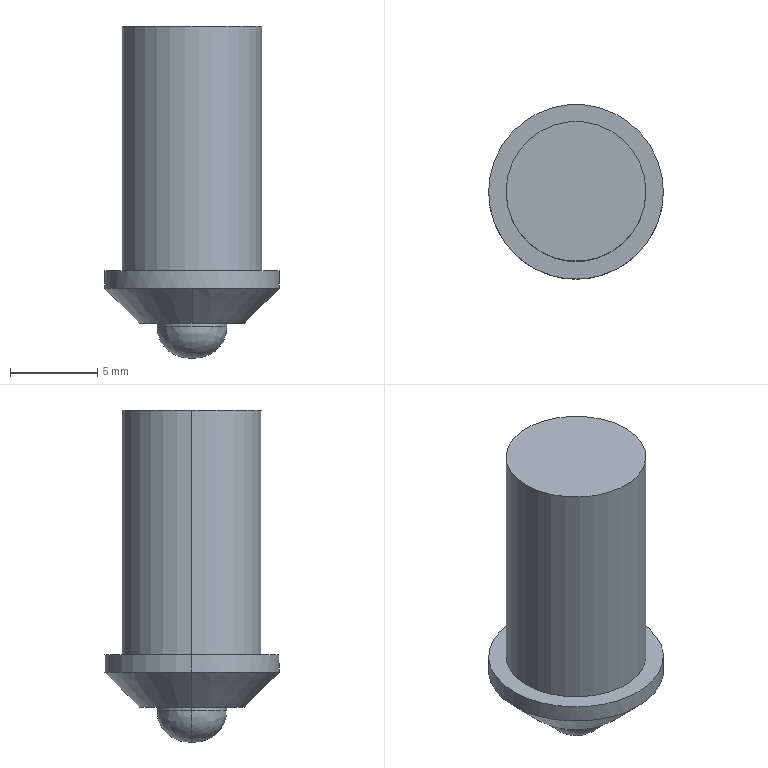Part | STEP file | 15V-DIANYUANZHISHIDENG.stp.STEP | 1 solid | 15 faces | box 10 x 10 x 19 mm | volume 903.03 mm3 | cylinder 6 | plane 4 | cone 3 | spline 2 | commonest cylinder face diameters 4 x2 8 x2 10 x2
STEP:
#1=CARTESIAN_POINT('',(0.2,0.,0.));
#2=VERTEX_POINT('',#1);
#3=CARTESIAN_POINT('',(-0.2,0.,0.));
#4=VERTEX_POINT('',#3);
#5=CARTESIAN_POINT('',(0.,0.,0.));
#6=DIRECTION('',(0.,0.,-1.));
#7=DIRECTION('',(1.,0.,0.));
#8=AXIS2_PLACEMENT_3D('',#5,#6,#7);
#9=CIRCLE('',#8,0.2);
#10=EDGE_CURVE('',#2,#4,#9,.T.);
#11=ORIENTED_EDGE('',*,*,#10,.T.);
#12=CARTESIAN_POINT('',(0.,0.,0.));
#13=DIRECTION('',(0.,0.,-1.));
#14=DIRECTION('',(-1.,0.,0.));
#15=AXIS2_PLACEMENT_3D('',#12,#13,#14);
#16=CIRCLE('',#15,0.2);
#17=EDGE_CURVE('',#4,#2,#16,.T.);
#18=ORIENTED_EDGE('',*,*,#17,.T.);
#19=EDGE_LOOP('',(#11,#18));
#20=FACE_OUTER_BOUND('',#19,.T.);
#21=CARTESIAN_POINT('',(0.,0.,0.));
#22=DIRECTION('',(0.,0.,1.));
#23=DIRECTION('',(1.,0.,0.));
#24=AXIS2_PLACEMENT_3D('',#21,#22,#23);
#25=PLANE('',#24);
#26=ADVANCED_FACE('',(#20),#25,.F.);
#27=CARTESIAN_POINT('',(-2.,0.,1.8));
#28=VERTEX_POINT('',#27);
#29=CARTESIAN_POINT('',(-0.2,0.,1.8));
#30=DIRECTION('',(0.,1.,0.));
#31=DIRECTION('',(0.,0.,-1.));
#32=AXIS2_PLACEMENT_3D('',#29,#30,#31);
#33=CIRCLE('',#32,1.8);
#34=EDGE_CURVE('',#4,#28,#33,.T.);
#35=ORIENTED_EDGE('',*,*,#34,.T.);
#36=CARTESIAN_POINT('',(2.,0.,1.8));
#37=VERTEX_POINT('',#36);
#38=CARTESIAN_POINT('',(0.,0.,1.8));
#39=DIRECTION('',(0.,0.,-1.));
#40=DIRECTION('',(-1.,0.,0.));
#41=AXIS2_PLACEMENT_3D('',#38,#39,#40);
#42=CIRCLE('',#41,2.);
#43=EDGE_CURVE('',#28,#37,#42,.T.);
#44=ORIENTED_EDGE('',*,*,#43,.T.);
#45=CARTESIAN_POINT('',(0.2,0.,1.8));
#46=DIRECTION('',(0.,-1.,0.));
#47=DIRECTION('',(0.,0.,-1.));
#48=AXIS2_PLACEMENT_3D('',#45,#46,#47);
#49=CIRCLE('',#48,1.8);
#50=EDGE_CURVE('',#2,#37,#49,.T.);
#51=ORIENTED_EDGE('',*,*,#50,.F.);
#52=ORIENTED_EDGE('',*,*,#17,.F.);
#53=EDGE_LOOP('',(#35,#44,#51,#52));
#54=FACE_OUTER_BOUND('',#53,.T.);
#55=CARTESIAN_POINT('',(0.142,-0.02032,0.0008882));
#56=CARTESIAN_POINT('',(1.238,-0.1771,-0.03391));
#57=CARTESIAN_POINT('',(2.013,-0.2881,0.7494));
#58=CARTESIAN_POINT('',(1.979,-0.2831,1.857));
#59=CARTESIAN_POINT('',(0.1553,0.07257,0.0008882));
#60=CARTESIAN_POINT('',(1.354,0.6326,-0.03391));
#61=CARTESIAN_POINT('',(2.202,1.029,0.7494));
#62=CARTESIAN_POINT('',(2.164,1.011,1.857));
#63=CARTESIAN_POINT('',(0.09383,0.1435,0.0008882));
#64=CARTESIAN_POINT('',(0.818,1.251,-0.03391));
#65=CARTESIAN_POINT('',(1.33,2.034,0.7494));
#66=CARTESIAN_POINT('',(1.308,1.999,1.857));
#67=CARTESIAN_POINT('',(0.000000002,0.1435,0.0008882));
#68=CARTESIAN_POINT('',(0.000000017,1.251,-0.03391));
#69=CARTESIAN_POINT('',(0.000000028,2.034,0.7494));
#70=CARTESIAN_POINT('',(0.000000028,1.999,1.857));
#71=CARTESIAN_POINT('',(-0.09383,0.1435,0.0008882));
#72=CARTESIAN_POINT('',(-0.818,1.251,-0.03391));
#73=CARTESIAN_POINT('',(-1.33,2.034,0.7494));
#74=CARTESIAN_POINT('',(-1.308,1.999,1.857));
#75=CARTESIAN_POINT('',(-0.1553,0.07257,0.0008882));
#76=CARTESIAN_POINT('',(-1.354,0.6326,-0.03391));
#77=CARTESIAN_POINT('',(-2.202,1.029,0.7494));
#78=CARTESIAN_POINT('',(-2.164,1.011,1.857));
#79=CARTESIAN_POINT('',(-0.142,-0.02032,0.0008882));
#80=CARTESIAN_POINT('',(-1.238,-0.1771,-0.03391));
#81=CARTESIAN_POINT('',(-2.013,-0.2881,0.7494));
#82=CARTESIAN_POINT('',(-1.979,-0.2831,1.857));
#83=(BOUNDED_SURFACE()B_SPLINE_SURFACE(3,3,((#55,#56,#57,#58),(#59,#60,#61,#62),(#63,#64,#65,#66),(#67,#68,#69,#70),(#71,#72,#73,#74),(#75,#76,#77,#78),(#79,#80,#81,#82)),.UNSPECIFIED.,.F.,.F.,.F.)B_SPLINE_SURFACE_WITH_KNOTS((4,3,4),(4,4),(0.,1.,2.),(0.,1.),.UNSPECIFIED.)GEOMETRIC_REPRESENTATION_ITEM()RATIONAL_B_SPLINE_SURFACE(((1.435,1.133,1.133,1.435),(1.105,0.8725,0.8725,1.105),(1.105,0.8725,0.8725,1.105),(1.435,1.133,1.133,1.435),(1.105,0.8725,0.8725,1.105),(1.105,0.8725,0.8725,1.105),(1.435,1.133,1.133,1.435)))REPRESENTATION_ITEM('')SURFACE());
#84=ADVANCED_FACE('',(#54),#83,.T.);
#85=ORIENTED_EDGE('',*,*,#50,.T.);
#86=CARTESIAN_POINT('',(0.,0.,1.8));
#87=DIRECTION('',(0.,0.,-1.));
#88=DIRECTION('',(1.,0.,0.));
#89=AXIS2_PLACEMENT_3D('',#86,#87,#88);
#90=CIRCLE('',#89,2.);
#91=EDGE_CURVE('',#37,#28,#90,.T.);
#92=ORIENTED_EDGE('',*,*,#91,.T.);
#93=ORIENTED_EDGE('',*,*,#34,.F.);
#94=ORIENTED_EDGE('',*,*,#10,.F.);
#95=EDGE_LOOP('',(#85,#92,#93,#94));
#96=FACE_OUTER_BOUND('',#95,.T.);
#97=CARTESIAN_POINT('',(-0.142,0.02032,0.0008882));
#98=CARTESIAN_POINT('',(-1.238,0.1771,-0.03391));
#99=CARTESIAN_POINT('',(-2.013,0.2881,0.7494));
#100=CARTESIAN_POINT('',(-1.979,0.2831,1.857));
#101=CARTESIAN_POINT('',(-0.1553,-0.07257,0.0008882));
#102=CARTESIAN_POINT('',(-1.354,-0.6326,-0.03391));
#103=CARTESIAN_POINT('',(-2.202,-1.029,0.7494));
#104=CARTESIAN_POINT('',(-2.164,-1.011,1.857));
#105=CARTESIAN_POINT('',(-0.09383,-0.1435,0.0008882));
#106=CARTESIAN_POINT('',(-0.818,-1.251,-0.03391));
#107=CARTESIAN_POINT('',(-1.33,-2.034,0.7494));
#108=CARTESIAN_POINT('',(-1.308,-1.999,1.857));
#109=CARTESIAN_POINT('',(-0.000000002,-0.1435,0.0008882));
#110=CARTESIAN_POINT('',(-0.000000017,-1.251,-0.03391));
#111=CARTESIAN_POINT('',(-0.000000028,-2.034,0.7494));
#112=CARTESIAN_POINT('',(-0.000000028,-1.999,1.857));
#113=CARTESIAN_POINT('',(0.09383,-0.1435,0.0008882));
#114=CARTESIAN_POINT('',(0.818,-1.251,-0.03391));
#115=CARTESIAN_POINT('',(1.33,-2.034,0.7494));
#116=CARTESIAN_POINT('',(1.308,-1.999,1.857));
#117=CARTESIAN_POINT('',(0.1553,-0.07257,0.0008882));
#118=CARTESIAN_POINT('',(1.354,-0.6326,-0.03391));
#119=CARTESIAN_POINT('',(2.202,-1.029,0.7494));
#120=CARTESIAN_POINT('',(2.164,-1.011,1.857));
#121=CARTESIAN_POINT('',(0.142,0.02032,0.0008882));
#122=CARTESIAN_POINT('',(1.238,0.1771,-0.03391));
#123=CARTESIAN_POINT('',(2.013,0.2881,0.7494));
#124=CARTESIAN_POINT('',(1.979,0.2831,1.857));
#125=(BOUNDED_SURFACE()B_SPLINE_SURFACE(3,3,((#97,#98,#99,#100),(#101,#102,#103,#104),(#105,#106,#107,#108),(#109,#110,#111,#112),(#113,#114,#115,#116),(#117,#118,#119,#120),(#121,#122,#123,#124)),.UNSPECIFIED.,.F.,.F.,.T.)B_SPLINE_SURFACE_WITH_KNOTS((4,3,4),(4,4),(0.,1.,2.),(0.,1.),.UNSPECIFIED.)GEOMETRIC_REPRESENTATION_ITEM()RATIONAL_B_SPLINE_SURFACE(((1.435,1.133,1.133,1.435),(1.105,0.8725,0.8725,1.105),(1.105,0.8725,0.8725,1.105),(1.435,1.133,1.133,1.435),(1.105,0.8725,0.8725,1.105),(1.105,0.8725,0.8725,1.105),(1.435,1.133,1.133,1.435)))REPRESENTATION_ITEM('')SURFACE());
#126=ADVANCED_FACE('',(#96),#125,.T.);
#127=CARTESIAN_POINT('',(2.,0.,2.));
#128=VERTEX_POINT('',#127);
#129=CARTESIAN_POINT('',(2.,0.,1.8));
#130=DIRECTION('',(0.,-0.000000001,1.));
#131=VECTOR('',#130,1000.);
#132=LINE('',#129,#131);
#133=EDGE_CURVE('',#37,#128,#132,.T.);
#134=ORIENTED_EDGE('',*,*,#133,.T.);
#135=CARTESIAN_POINT('',(-2.,0.,2.));
#136=VERTEX_POINT('',#135);
#137=CARTESIAN_POINT('',(0.,0.,2.));
#138=DIRECTION('',(0.,0.,1.));
#139=DIRECTION('',(-1.,0.,0.));
#140=AXIS2_PLACEMENT_3D('',#137,#138,#139);
#141=CIRCLE('',#140,2.);
#142=EDGE_CURVE('',#136,#128,#141,.T.);
#143=ORIENTED_EDGE('',*,*,#142,.F.);
#144=CARTESIAN_POINT('',(-2.,0.,1.8));
#145=DIRECTION('',(0.,0.000000001,1.));
#146=VECTOR('',#145,1000.);
#147=LINE('',#144,#146);
#148=EDGE_CURVE('',#28,#136,#147,.T.);
#149=ORIENTED_EDGE('',*,*,#148,.F.);
#150=ORIENTED_EDGE('',*,*,#91,.F.);
#151=EDGE_LOOP('',(#134,#143,#149,#150));
#152=FACE_OUTER_BOUND('',#151,.T.);
#153=CARTESIAN_POINT('',(0.,0.,0.));
#154=DIRECTION('',(0.,0.,1.));
#155=DIRECTION('',(1.,0.,0.));
#156=AXIS2_PLACEMENT_3D('',#153,#154,#155);
#157=CYLINDRICAL_SURFACE('',#156,2.);
#158=ADVANCED_FACE('',(#152),#157,.T.);
#159=ORIENTED_EDGE('',*,*,#148,.T.);
#160=CARTESIAN_POINT('',(0.,0.,2.));
#161=DIRECTION('',(0.,0.,1.));
#162=DIRECTION('',(1.,0.,0.));
#163=AXIS2_PLACEMENT_3D('',#160,#161,#162);
#164=CIRCLE('',#163,2.);
#165=EDGE_CURVE('',#128,#136,#164,.T.);
#166=ORIENTED_EDGE('',*,*,#165,.F.);
#167=ORIENTED_EDGE('',*,*,#133,.F.);
#168=ORIENTED_EDGE('',*,*,#43,.F.);
#169=EDGE_LOOP('',(#159,#166,#167,#168));
#170=FACE_OUTER_BOUND('',#169,.T.);
#171=CARTESIAN_POINT('',(0.,0.,0.));
#172=DIRECTION('',(0.,0.,1.));
#173=DIRECTION('',(1.,0.,0.));
#174=AXIS2_PLACEMENT_3D('',#171,#172,#173);
#175=CYLINDRICAL_SURFACE('',#174,2.);
#176=ADVANCED_FACE('',(#170),#175,.T.);
#177=ORIENTED_EDGE('',*,*,#142,.T.);
#178=ORIENTED_EDGE('',*,*,#165,.T.);
#179=EDGE_LOOP('',(#177,#178));
#180=FACE_BOUND('',#179,.T.);
#181=CARTESIAN_POINT('',(3.,0.,2.));
#182=VERTEX_POINT('',#181);
#183=CARTESIAN_POINT('',(0.,-3.,2.));
#184=VERTEX_POINT('',#183);
#185=CARTESIAN_POINT('',(0.,0.,2.));
#186=DIRECTION('',(0.,0.,-1.));
#187=DIRECTION('',(1.,0.,0.));
#188=AXIS2_PLACEMENT_3D('',#185,#186,#187);
#189=CIRCLE('',#188,3.);
#190=EDGE_CURVE('',#182,#184,#189,.T.);
#191=ORIENTED_EDGE('',*,*,#190,.T.);
#192=CARTESIAN_POINT('',(-3.,0.,2.));
#193=VERTEX_POINT('',#192);
#194=CARTESIAN_POINT('',(0.,0.,2.));
#195=DIRECTION('',(0.,0.,-1.));
#196=DIRECTION('',(1.,0.,0.));
#197=AXIS2_PLACEMENT_3D('',#194,#195,#196);
#198=CIRCLE('',#197,3.);
#199=EDGE_CURVE('',#184,#193,#198,.T.);
#200=ORIENTED_EDGE('',*,*,#199,.T.);
#201=CARTESIAN_POINT('',(0.,0.,2.));
#202=DIRECTION('',(0.,0.,-1.));
#203=DIRECTION('',(-1.,0.,0.));
#204=AXIS2_PLACEMENT_3D('',#201,#202,#203);
#205=CIRCLE('',#204,3.);
#206=EDGE_CURVE('',#193,#182,#205,.T.);
#207=ORIENTED_EDGE('',*,*,#206,.T.);
#208=EDGE_LOOP('',(#191,#200,#207));
#209=FACE_OUTER_BOUND('',#208,.T.);
#210=CARTESIAN_POINT('',(0.,0.,2.));
#211=DIRECTION('',(0.,0.,1.));
#212=DIRECTION('',(1.,0.,0.));
#213=AXIS2_PLACEMENT_3D('',#210,#211,#212);
#214=PLANE('',#213);
#215=ADVANCED_FACE('',(#180,#209),#214,.F.);
#216=CARTESIAN_POINT('',(-5.,0.,4.));
#217=VERTEX_POINT('',#216);
#218=CARTESIAN_POINT('',(-3.,0.,2.));
#219=DIRECTION('',(-0.7071,0.,0.7071));
#220=VECTOR('',#219,1000.);
#221=LINE('',#218,#220);
#222=EDGE_CURVE('',#193,#217,#221,.T.);
#223=ORIENTED_EDGE('',*,*,#222,.T.);
#224=CARTESIAN_POINT('',(5.,0.,4.));
#225=VERTEX_POINT('',#224);
#226=CARTESIAN_POINT('',(0.,0.,4.));
#227=DIRECTION('',(0.,0.,-1.));
#228=DIRECTION('',(-1.,0.,0.));
#229=AXIS2_PLACEMENT_3D('',#226,#227,#228);
#230=CIRCLE('',#229,5.);
#231=EDGE_CURVE('',#217,#225,#230,.T.);
#232=ORIENTED_EDGE('',*,*,#231,.T.);
#233=CARTESIAN_POINT('',(3.,0.,2.));
#234=DIRECTION('',(0.7071,0.,0.7071));
#235=VECTOR('',#234,1000.);
#236=LINE('',#233,#235);
#237=EDGE_CURVE('',#182,#225,#236,.T.);
#238=ORIENTED_EDGE('',*,*,#237,.F.);
#239=ORIENTED_EDGE('',*,*,#206,.F.);
#240=EDGE_LOOP('',(#223,#232,#238,#239));
#241=FACE_OUTER_BOUND('',#240,.T.);
#242=CARTESIAN_POINT('',(0.,0.,3.));
#243=DIRECTION('',(0.,0.,1.));
#244=DIRECTION('',(0.,-1.,0.));
#245=AXIS2_PLACEMENT_3D('',#242,#243,#244);
#246=CONICAL_SURFACE('',#245,4.,0.7854);
#247=ADVANCED_FACE('',(#241),#246,.T.);
#248=CARTESIAN_POINT('',(0.,-5.,4.));
#249=VERTEX_POINT('',#248);
#250=CARTESIAN_POINT('',(0.,-4.,3.));
#251=DIRECTION('',(0.,-0.7071,0.7071));
#252=VECTOR('',#251,1000.);
#253=LINE('',#250,#252);
#254=EDGE_CURVE('',#184,#249,#253,.T.);
#255=ORIENTED_EDGE('',*,*,#254,.F.);
#256=ORIENTED_EDGE('',*,*,#190,.F.);
#257=ORIENTED_EDGE('',*,*,#237,.T.);
#258=CARTESIAN_POINT('',(0.,0.,4.));
#259=DIRECTION('',(0.,0.,-1.));
#260=DIRECTION('',(1.,0.,0.));
#261=AXIS2_PLACEMENT_3D('',#258,#259,#260);
#262=CIRCLE('',#261,5.);
#263=EDGE_CURVE('',#225,#249,#262,.T.);
#264=ORIENTED_EDGE('',*,*,#263,.T.);
#265=EDGE_LOOP('',(#255,#256,#257,#264));
#266=FACE_OUTER_BOUND('',#265,.T.);
#267=CARTESIAN_POINT('',(0.,0.,3.));
#268=DIRECTION('',(0.,0.,1.));
#269=DIRECTION('',(0.,-1.,0.));
#270=AXIS2_PLACEMENT_3D('',#267,#268,#269);
#271=CONICAL_SURFACE('',#270,4.,0.7854);
#272=ADVANCED_FACE('',(#266),#271,.T.);
#273=CARTESIAN_POINT('',(5.,0.,5.));
#274=VERTEX_POINT('',#273);
#275=CARTESIAN_POINT('',(5.,0.,4.));
#276=DIRECTION('',(-0.000000281,0.,1.));
#277=VECTOR('',#276,1000.);
#278=LINE('',#275,#277);
#279=EDGE_CURVE('',#225,#274,#278,.T.);
#280=ORIENTED_EDGE('',*,*,#279,.T.);
#281=CARTESIAN_POINT('',(-5.,0.,5.));
#282=VERTEX_POINT('',#281);
#283=CARTESIAN_POINT('',(0.,0.,5.));
#284=DIRECTION('',(0.,0.,1.));
#285=DIRECTION('',(-1.,0.,0.));
#286=AXIS2_PLACEMENT_3D('',#283,#284,#285);
#287=CIRCLE('',#286,5.);
#288=EDGE_CURVE('',#282,#274,#287,.T.);
#289=ORIENTED_EDGE('',*,*,#288,.F.);
#290=CARTESIAN_POINT('',(-5.,0.,4.));
#291=DIRECTION('',(0.000000281,0.,1.));
#292=VECTOR('',#291,1000.);
#293=LINE('',#290,#292);
#294=EDGE_CURVE('',#217,#282,#293,.T.);
#295=ORIENTED_EDGE('',*,*,#294,.F.);
#296=CARTESIAN_POINT('',(0.,0.,4.));
#297=DIRECTION('',(0.,0.,-1.));
#298=DIRECTION('',(1.,0.,0.));
#299=AXIS2_PLACEMENT_3D('',#296,#297,#298);
#300=CIRCLE('',#299,5.);
#301=EDGE_CURVE('',#249,#217,#300,.T.);
#302=ORIENTED_EDGE('',*,*,#301,.F.);
#303=ORIENTED_EDGE('',*,*,#263,.F.);
#304=EDGE_LOOP('',(#280,#289,#295,#302,#303));
#305=FACE_OUTER_BOUND('',#304,.T.);
#306=CARTESIAN_POINT('',(0.,0.,2.));
#307=DIRECTION('',(0.,0.,1.));
#308=DIRECTION('',(1.,0.,0.));
#309=AXIS2_PLACEMENT_3D('',#306,#307,#308);
#310=CYLINDRICAL_SURFACE('',#309,5.);
#311=ADVANCED_FACE('',(#305),#310,.T.);
#312=ORIENTED_EDGE('',*,*,#294,.T.);
#313=CARTESIAN_POINT('',(0.,0.,5.));
#314=DIRECTION('',(0.,0.,1.));
#315=DIRECTION('',(1.,0.,0.));
#316=AXIS2_PLACEMENT_3D('',#313,#314,#315);
#317=CIRCLE('',#316,5.);
#318=EDGE_CURVE('',#274,#282,#317,.T.);
#319=ORIENTED_EDGE('',*,*,#318,.F.);
#320=ORIENTED_EDGE('',*,*,#279,.F.);
#321=ORIENTED_EDGE('',*,*,#231,.F.);
#322=EDGE_LOOP('',(#312,#319,#320,#321));
#323=FACE_OUTER_BOUND('',#322,.T.);
#324=CARTESIAN_POINT('',(0.,0.,2.));
#325=DIRECTION('',(0.,0.,1.));
#326=DIRECTION('',(1.,0.,0.));
#327=AXIS2_PLACEMENT_3D('',#324,#325,#326);
#328=CYLINDRICAL_SURFACE('',#327,5.);
#329=ADVANCED_FACE('',(#323),#328,.T.);
#330=CARTESIAN_POINT('',(-4.,0.,5.));
#331=VERTEX_POINT('',#330);
#332=CARTESIAN_POINT('',(4.,0.,5.));
#333=VERTEX_POINT('',#332);
#334=CARTESIAN_POINT('',(0.,0.,5.));
#335=DIRECTION('',(0.,0.,1.));
#336=DIRECTION('',(-1.,0.,0.));
#337=AXIS2_PLACEMENT_3D('',#334,#335,#336);
#338=CIRCLE('',#337,4.);
#339=EDGE_CURVE('',#331,#333,#338,.T.);
#340=ORIENTED_EDGE('',*,*,#339,.F.);
#341=CARTESIAN_POINT('',(0.,0.,5.));
#342=DIRECTION('',(0.,0.,1.));
#343=DIRECTION('',(1.,0.,0.));
#344=AXIS2_PLACEMENT_3D('',#341,#342,#343);
#345=CIRCLE('',#344,4.);
#346=EDGE_CURVE('',#333,#331,#345,.T.);
#347=ORIENTED_EDGE('',*,*,#346,.F.);
#348=EDGE_LOOP('',(#340,#347));
#349=FACE_BOUND('',#348,.T.);
#350=ORIENTED_EDGE('',*,*,#288,.T.);
#351=ORIENTED_EDGE('',*,*,#318,.T.);
#352=EDGE_LOOP('',(#350,#351));
#353=FACE_OUTER_BOUND('',#352,.T.);
#354=CARTESIAN_POINT('',(0.,0.,5.));
#355=DIRECTION('',(0.,0.,1.));
#356=DIRECTION('',(1.,0.,0.));
#357=AXIS2_PLACEMENT_3D('',#354,#355,#356);
#358=PLANE('',#357);
#359=ADVANCED_FACE('',(#349,#353),#358,.T.);
#360=CARTESIAN_POINT('',(-4.,0.,19.));
#361=VERTEX_POINT('',#360);
#362=CARTESIAN_POINT('',(-4.,0.,5.));
#363=DIRECTION('',(0.,0.,1.));
#364=VECTOR('',#363,1000.);
#365=LINE('',#362,#364);
#366=EDGE_CURVE('',#331,#361,#365,.T.);
#367=ORIENTED_EDGE('',*,*,#366,.T.);
#368=CARTESIAN_POINT('',(4.,0.,19.));
#369=VERTEX_POINT('',#368);
#370=CARTESIAN_POINT('',(0.,0.,19.));
#371=DIRECTION('',(0.,0.,1.));
#372=DIRECTION('',(1.,0.,0.));
#373=AXIS2_PLACEMENT_3D('',#370,#371,#372);
#374=CIRCLE('',#373,4.);
#375=EDGE_CURVE('',#369,#361,#374,.T.);
#376=ORIENTED_EDGE('',*,*,#375,.F.);
#377=CARTESIAN_POINT('',(4.,0.,5.));
#378=DIRECTION('',(0.,0.,1.));
#379=VECTOR('',#378,1000.);
#380=LINE('',#377,#379);
#381=EDGE_CURVE('',#333,#369,#380,.T.);
#382=ORIENTED_EDGE('',*,*,#381,.F.);
#383=ORIENTED_EDGE('',*,*,#346,.T.);
#384=EDGE_LOOP('',(#367,#376,#382,#383));
#385=FACE_OUTER_BOUND('',#384,.T.);
#386=CARTESIAN_POINT('',(0.,0.,5.));
#387=DIRECTION('',(0.,0.,1.));
#388=DIRECTION('',(1.,0.,0.));
#389=AXIS2_PLACEMENT_3D('',#386,#387,#388);
#390=CYLINDRICAL_SURFACE('',#389,4.);
#391=ADVANCED_FACE('',(#385),#390,.T.);
#392=ORIENTED_EDGE('',*,*,#381,.T.);
#393=CARTESIAN_POINT('',(0.,0.,19.));
#394=DIRECTION('',(0.,0.,1.));
#395=DIRECTION('',(-1.,0.,0.));
#396=AXIS2_PLACEMENT_3D('',#393,#394,#395);
#397=CIRCLE('',#396,4.);
#398=EDGE_CURVE('',#361,#369,#397,.T.);
#399=ORIENTED_EDGE('',*,*,#398,.F.);
#400=ORIENTED_EDGE('',*,*,#366,.F.);
#401=ORIENTED_EDGE('',*,*,#339,.T.);
#402=EDGE_LOOP('',(#392,#399,#400,#401));
#403=FACE_OUTER_BOUND('',#402,.T.);
#404=CARTESIAN_POINT('',(0.,0.,5.));
#405=DIRECTION('',(0.,0.,1.));
#406=DIRECTION('',(1.,0.,0.));
#407=AXIS2_PLACEMENT_3D('',#404,#405,#406);
#408=CYLINDRICAL_SURFACE('',#407,4.);
#409=ADVANCED_FACE('',(#403),#408,.T.);
#410=ORIENTED_EDGE('',*,*,#398,.T.);
#411=ORIENTED_EDGE('',*,*,#375,.T.);
#412=EDGE_LOOP('',(#410,#411));
#413=FACE_OUTER_BOUND('',#412,.T.);
#414=CARTESIAN_POINT('',(0.,0.,19.));
#415=DIRECTION('',(0.,0.,1.));
#416=DIRECTION('',(1.,0.,0.));
#417=AXIS2_PLACEMENT_3D('',#414,#415,#416);
#418=PLANE('',#417);
#419=ADVANCED_FACE('',(#413),#418,.T.);
#420=ORIENTED_EDGE('',*,*,#199,.F.);
#421=ORIENTED_EDGE('',*,*,#254,.T.);
#422=ORIENTED_EDGE('',*,*,#301,.T.);
#423=ORIENTED_EDGE('',*,*,#222,.F.);
#424=EDGE_LOOP('',(#420,#421,#422,#423));
#425=FACE_OUTER_BOUND('',#424,.T.);
#426=CARTESIAN_POINT('',(0.,0.,3.));
#427=DIRECTION('',(0.,0.,1.));
#428=DIRECTION('',(0.,-1.,0.));
#429=AXIS2_PLACEMENT_3D('',#426,#427,#428);
#430=CONICAL_SURFACE('',#429,4.,0.7854);
#431=ADVANCED_FACE('',(#425),#430,.T.);
#432=CLOSED_SHELL('',(#26,#84,#126,#158,#176,#215,#247,#272,#311,#329,#359,#391,#409,#419,#431));
#433=MANIFOLD_SOLID_BREP('',#432);
#434=CARTESIAN_POINT('',(0.,0.,0.));
#435=DIRECTION('',(0.,0.,1.));
#436=DIRECTION('',(1.,0.,0.));
#437=AXIS2_PLACEMENT_3D('',#434,#435,#436);
#438=(LENGTH_UNIT()NAMED_UNIT(*)SI_UNIT(.MILLI.,.METRE.));
#439=UNCERTAINTY_MEASURE_WITH_UNIT(LENGTH_MEASURE(0.00001),#438,'','');
#440=(NAMED_UNIT(*)PLANE_ANGLE_UNIT()SI_UNIT($,.RADIAN.));
#441=(NAMED_UNIT(*)SI_UNIT($,.STERADIAN.)SOLID_ANGLE_UNIT());
#442=(GEOMETRIC_REPRESENTATION_CONTEXT(3)GLOBAL_UNCERTAINTY_ASSIGNED_CONTEXT((#439))GLOBAL_UNIT_ASSIGNED_CONTEXT((#438,#440,#441))REPRESENTATION_CONTEXT('',''));
#443=ADVANCED_BREP_SHAPE_REPRESENTATION('',(#433,#437),#442);